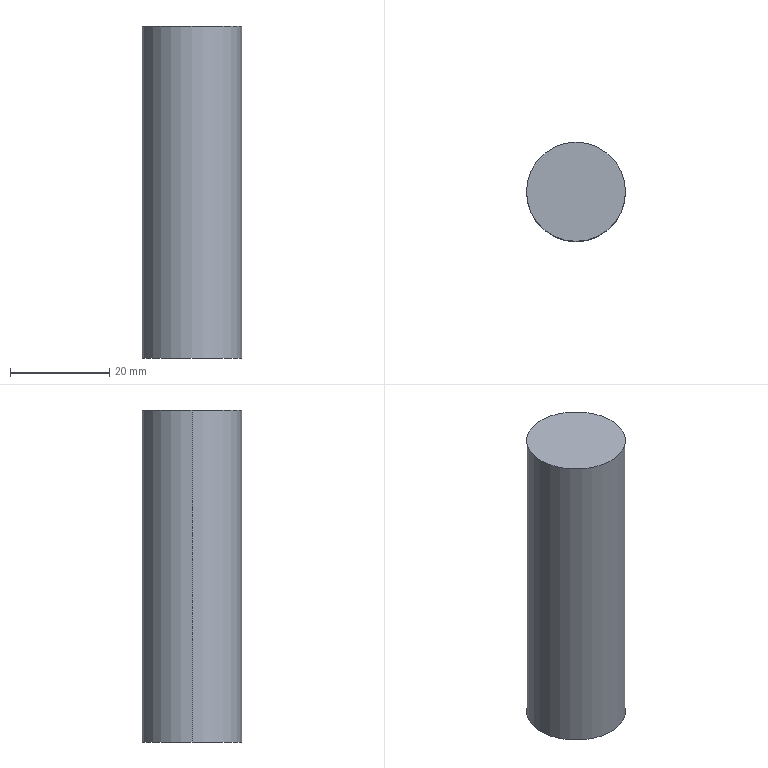Part | Creo | 1 solid | 4 faces | box 20 x 20 x 67 mm | volume 21049 mm3 | cylinder 2 | plane 2 | commonest cylinder face diameters 20 x2
STEP:
#1=CARTESIAN_POINT('',(0.,0.,0.));
#2=DIRECTION('',(0.,0.,1.));
#3=DIRECTION('',(1.,0.,0.));
#4=AXIS2_PLACEMENT_3D('',#1,#2,#3);
#5=CARTESIAN_POINT('',(-195.878,150.543,223.245));
#6=VERTEX_POINT('',#5);
#7=CARTESIAN_POINT('',(-175.878,150.543,223.245));
#8=VERTEX_POINT('',#7);
#9=CARTESIAN_POINT('',(-185.878,150.543,223.245));
#10=DIRECTION('',(0.,0.,-1.));
#11=DIRECTION('',(-1.,0.,0.));
#12=AXIS2_PLACEMENT_3D('',#9,#10,#11);
#13=CIRCLE('',#12,10.);
#14=EDGE_CURVE('',#6,#8,#13,.T.);
#15=ORIENTED_EDGE('',*,*,#14,.T.);
#16=CARTESIAN_POINT('',(-175.878,150.543,290.245));
#17=VERTEX_POINT('',#16);
#18=CARTESIAN_POINT('',(-175.878,150.543,223.245));
#19=DIRECTION('',(0.,0.,1.));
#20=VECTOR('',#19,67.);
#21=LINE('',#18,#20);
#22=EDGE_CURVE('',#8,#17,#21,.T.);
#23=ORIENTED_EDGE('',*,*,#22,.T.);
#24=CARTESIAN_POINT('',(-195.878,150.543,290.245));
#25=VERTEX_POINT('',#24);
#26=CARTESIAN_POINT('',(-185.878,150.543,290.245));
#27=DIRECTION('',(0.,0.,1.));
#28=DIRECTION('',(1.,0.,0.));
#29=AXIS2_PLACEMENT_3D('',#26,#27,#28);
#30=CIRCLE('',#29,10.);
#31=EDGE_CURVE('',#17,#25,#30,.T.);
#32=ORIENTED_EDGE('',*,*,#31,.T.);
#33=CARTESIAN_POINT('',(-195.878,150.543,223.245));
#34=DIRECTION('',(0.,0.,1.));
#35=VECTOR('',#34,67.);
#36=LINE('',#33,#35);
#37=EDGE_CURVE('',#6,#25,#36,.T.);
#38=ORIENTED_EDGE('',*,*,#37,.F.);
#39=EDGE_LOOP('',(#15,#23,#32,#38));
#40=FACE_OUTER_BOUND('',#39,.F.);
#41=CARTESIAN_POINT('',(-185.878,150.543,224.245));
#42=DIRECTION('',(0.,0.,1.));
#43=DIRECTION('',(1.,0.,0.));
#44=AXIS2_PLACEMENT_3D('',#41,#42,#43);
#45=CYLINDRICAL_SURFACE('',#44,10.);
#46=ADVANCED_FACE('',(#40),#45,.T.);
#47=ORIENTED_EDGE('',*,*,#14,.F.);
#48=CARTESIAN_POINT('',(-185.878,150.543,223.245));
#49=DIRECTION('',(0.,0.,-1.));
#50=DIRECTION('',(1.,0.,0.));
#51=AXIS2_PLACEMENT_3D('',#48,#49,#50);
#52=CIRCLE('',#51,10.);
#53=EDGE_CURVE('',#8,#6,#52,.T.);
#54=ORIENTED_EDGE('',*,*,#53,.F.);
#55=EDGE_LOOP('',(#47,#54));
#56=FACE_OUTER_BOUND('',#55,.F.);
#57=CARTESIAN_POINT('',(-185.878,150.543,223.245));
#58=DIRECTION('',(0.,0.,1.));
#59=DIRECTION('',(1.,0.,0.));
#60=AXIS2_PLACEMENT_3D('',#57,#58,#59);
#61=PLANE('',#60);
#62=ADVANCED_FACE('',(#56),#61,.F.);
#63=ORIENTED_EDGE('',*,*,#53,.T.);
#64=ORIENTED_EDGE('',*,*,#37,.T.);
#65=CARTESIAN_POINT('',(-185.878,150.543,290.245));
#66=DIRECTION('',(0.,0.,1.));
#67=DIRECTION('',(-1.,0.,0.));
#68=AXIS2_PLACEMENT_3D('',#65,#66,#67);
#69=CIRCLE('',#68,10.);
#70=EDGE_CURVE('',#25,#17,#69,.T.);
#71=ORIENTED_EDGE('',*,*,#70,.T.);
#72=ORIENTED_EDGE('',*,*,#22,.F.);
#73=EDGE_LOOP('',(#63,#64,#71,#72));
#74=FACE_OUTER_BOUND('',#73,.F.);
#75=CARTESIAN_POINT('',(-185.878,150.543,224.245));
#76=DIRECTION('',(0.,0.,1.));
#77=DIRECTION('',(1.,0.,0.));
#78=AXIS2_PLACEMENT_3D('',#75,#76,#77);
#79=CYLINDRICAL_SURFACE('',#78,10.);
#80=ADVANCED_FACE('',(#74),#79,.T.);
#81=ORIENTED_EDGE('',*,*,#70,.F.);
#82=ORIENTED_EDGE('',*,*,#31,.F.);
#83=EDGE_LOOP('',(#81,#82));
#84=FACE_OUTER_BOUND('',#83,.F.);
#85=CARTESIAN_POINT('',(-185.878,150.543,290.245));
#86=DIRECTION('',(0.,0.,1.));
#87=DIRECTION('',(1.,0.,0.));
#88=AXIS2_PLACEMENT_3D('',#85,#86,#87);
#89=PLANE('',#88);
#90=ADVANCED_FACE('',(#84),#89,.T.);
#91=CLOSED_SHELL('',(#46,#62,#80,#90));
#92=MANIFOLD_SOLID_BREP('',#91);
#93=(LENGTH_UNIT()NAMED_UNIT(*)SI_UNIT(.MILLI.,.METRE.));
#94=UNCERTAINTY_MEASURE_WITH_UNIT(LENGTH_MEASURE(0.007272),#93,'','');
#95=(NAMED_UNIT(*)PLANE_ANGLE_UNIT()SI_UNIT($,.RADIAN.));
#96=PLANE_ANGLE_MEASURE_WITH_UNIT(PLANE_ANGLE_MEASURE(0.01745),#95);
#97=(CONVERSION_BASED_UNIT('DEGREE',#96)NAMED_UNIT(*)PLANE_ANGLE_UNIT());
#98=(NAMED_UNIT(*)SI_UNIT($,.STERADIAN.)SOLID_ANGLE_UNIT());
#99=(GEOMETRIC_REPRESENTATION_CONTEXT(3)GLOBAL_UNCERTAINTY_ASSIGNED_CONTEXT((#94))GLOBAL_UNIT_ASSIGNED_CONTEXT((#93,#97,#98))REPRESENTATION_CONTEXT('',''));
#100=ADVANCED_BREP_SHAPE_REPRESENTATION('',(#4,#92),#99);